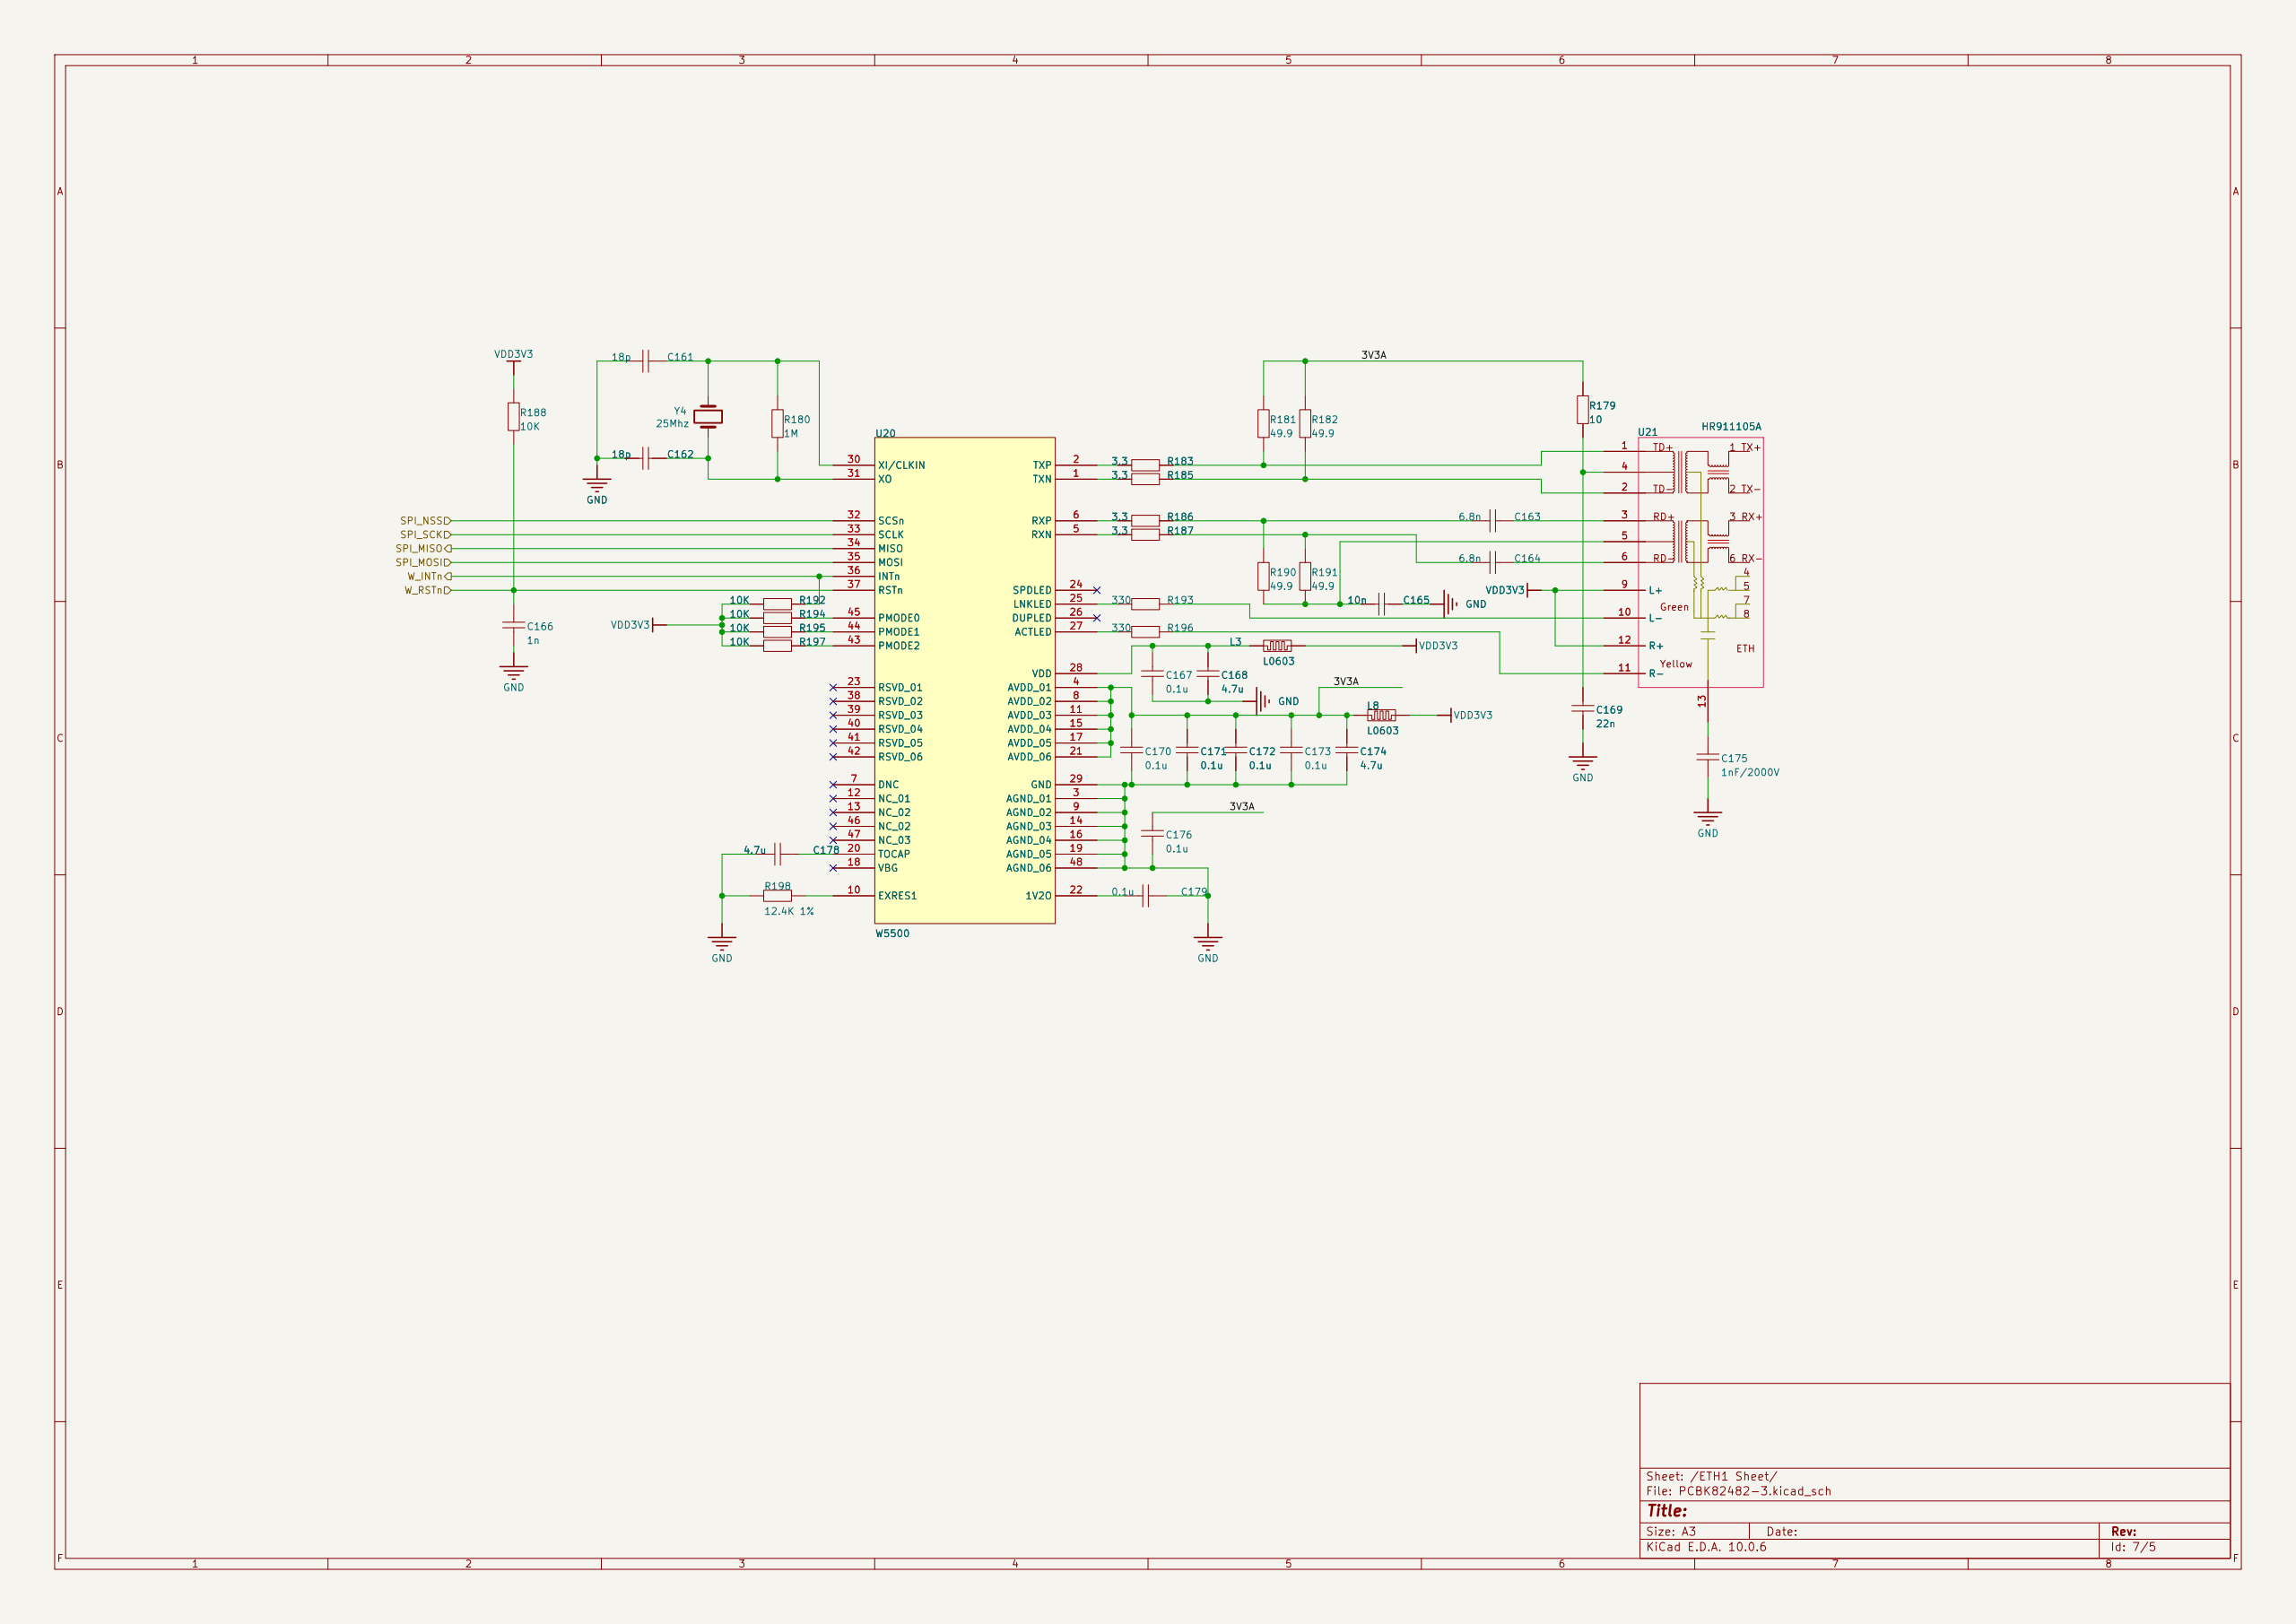Circuit board | KiCad | 154 parts | 201 nets | one sheet of the schematic
Parts on this sheet (reference | value | footprint):
C161 | 18p | Library:C0603
C162 | 18p | Library:C0603
C163 | 6.8n | Library:C0603
C164 | 6.8n | Library:C0603
C165 | 10n | Library:C0603
C166 | 1n | Library:C0603
C167 | 0.1u | Library:C0603
C168 | 4.7u | Library:C0603
C169 | 22n | Library:C0603
C170
C171
C172
C173
C174 | 4.7u | Library:C0603
C175 | 1nF/2000V | Library:C1808
C176 | 0.1u | Library:C0603
C178 | 4.7u | Library:C0603
C179 | 0.1u | Library:C0603
L3
L8 | L0603 | Library:L0603
R179 | 10 | Library:R0603
R180 | 1M | Library:R0603
R181 | 49.9 | Library:R0603
R182 | 49.9 | Library:R0603
R183 | 3.3 | Library:R0603
R185
R186
R187
R190 | 49.9 | Library:R0603
R191 | 49.9 | Library:R0603
R192 | 10K | Library:R0603
R193 | 330 | Library:R0603
R194 | 10K | Library:R0603
R195 | 10K | Library:R0603
R196 | 330 | Library:R0603
R197 | 10K | Library:R0603
R198 | 12.4K 1% | Library:R0603
U20 | W5500 | Library:P48LQFP
U21 | HR911105A | Library:HR911105A
Y4 | 25Mhz | Crystal:Crystal_SMD_5032-2Pin_5.0x3.2mm_HandSoldering
Nets of these parts (net: part-pin ...):
/ETH1 Sheet/3V3A: C170-2 C171-2 C172-2 C173-2 C174-2 C176-2 L8-1 R179-1 R181-1 R182-1 U20-4 U20-8 U20-11 U20-15 U20-17 U20-21
/Vision_Interface/BTB_P400: R192-1 U20-36
/Vision_Interface/BTB_P710: C166-2 U20-37
GND: C161-2 C162-2 C165-1 C166-1 C167-1 C168-1 C169-2 C170-1 C171-1 C172-1 C173-1 C174-1 C175-1 C176-1 C178-2 C179-1 R198-2 U20-3 U20-9 U20-14 U20-16 U20-19 U20-29 U20-48
Net-(C163-Pad1): C163-1 U21-3
Net-(C163-Pad2): C163-2 R186-1 R190-1
Net-(C164-Pad1): C164-1 U21-6
Net-(C164-Pad2): C164-2 R187-1 R191-1
Net-(C165-Pad2): C165-2 R190-2 R191-2 U21-5
Net-(C169-Pad1): C169-1 R179-2 U21-4
Net-(C175-Pad2): C175-2 U21-13
Net-(R181-Pad2): R181-2 R183-1 U21-1
Net-(R182-Pad2): R182-2 R185-1 U21-2
Net-(U20-1V2O): C179-2 U20-22
Net-(U20-ACTLED): R196-2 U20-27
Net-(U20-EXRES1): R198-1 U20-10
Net-(U20-LNKLED): R193-2 U20-25
Net-(U20-PMODE0): R194-1 U20-45
Net-(U20-PMODE1): R195-1 U20-44
Net-(U20-PMODE2): R197-1 U20-43
Net-(U20-RXN): R187-2 U20-5
Net-(U20-RXP): R186-2 U20-6
Net-(U20-TOCAP): C178-1 U20-20
Net-(U20-TXN): R185-2 U20-1
Net-(U20-TXP): R183-2 U20-2
Net-(U20-VDD): C167-2 C168-2 L3-1 U20-28
Net-(U20-XI{slash}CLKIN): C161-1 R180-1 Y4-2 U20-30
Net-(U20-XO): C162-1 R180-2 Y4-1 U20-31
Net-(U21-L-): R193-1 U21-10
Net-(U21-R-): R196-1 U21-11
VDD3V3: L3-2 L8-2 R192-2 R194-2 R195-2 R197-2 U21-9 U21-12